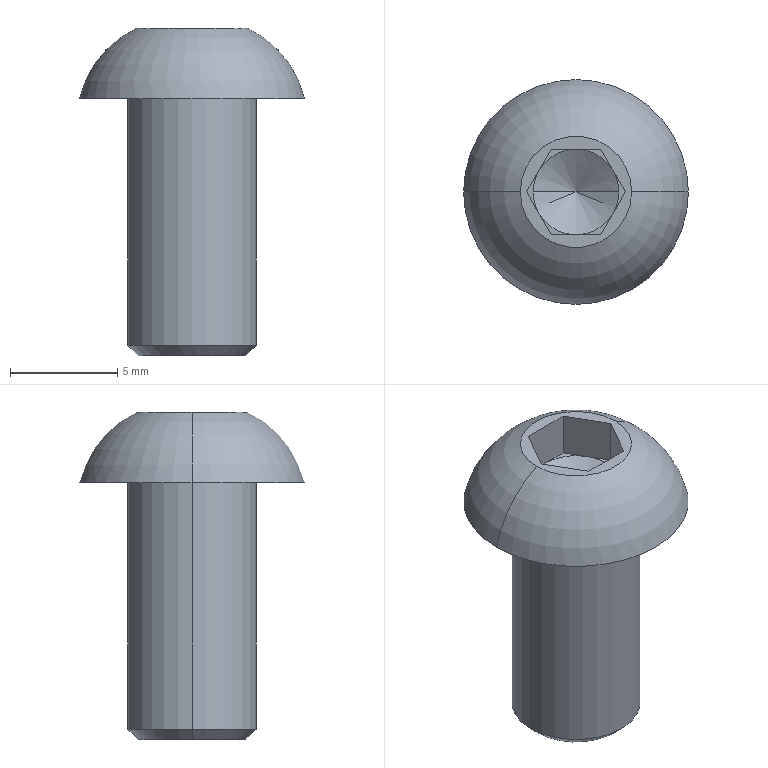Part | NX | features BREP 1 | 1 solid | 23 faces | box 10.5 x 10.5 x 15.3 mm | volume 504.847 mm3 | plane 15 | cone 4 | torus 2 | cylinder 2 | commonest cylinder face diameters 6 x2
STEP:
#1=CARTESIAN_POINT('',(0.,0.,0.0453));
#2=VERTEX_POINT('',#1);
#3=CARTESIAN_POINT('',(-2.,0.,1.2));
#4=VERTEX_POINT('',#3);
#5=CARTESIAN_POINT('',(-2.,0.,1.2));
#6=DIRECTION('',(-0.866,0.,0.5));
#7=VECTOR('',#6,1000.);
#8=LINE('',#5,#7);
#9=EDGE_CURVE('',#2,#4,#8,.T.);
#10=ORIENTED_EDGE('',*,*,#9,.F.);
#11=CARTESIAN_POINT('',(2.,0.,1.2));
#12=VERTEX_POINT('',#11);
#13=CARTESIAN_POINT('',(2.,0.,1.2));
#14=DIRECTION('',(0.866,0.,0.5));
#15=VECTOR('',#14,1000.);
#16=LINE('',#13,#15);
#17=EDGE_CURVE('',#2,#12,#16,.T.);
#18=ORIENTED_EDGE('',*,*,#17,.T.);
#19=CARTESIAN_POINT('',(1.732,1.,1.2));
#20=VERTEX_POINT('',#19);
#21=CARTESIAN_POINT('',(0.,0.,1.2));
#22=DIRECTION('',(0.,0.,1.));
#23=DIRECTION('',(1.,0.,0.));
#24=AXIS2_PLACEMENT_3D('',#21,#22,#23);
#25=CIRCLE('',#24,2.);
#26=EDGE_CURVE('',#12,#20,#25,.T.);
#27=ORIENTED_EDGE('',*,*,#26,.T.);
#28=CARTESIAN_POINT('',(0.,2.,1.2));
#29=VERTEX_POINT('',#28);
#30=CARTESIAN_POINT('',(0.,0.,1.2));
#31=DIRECTION('',(0.,0.,1.));
#32=DIRECTION('',(1.,0.,0.));
#33=AXIS2_PLACEMENT_3D('',#30,#31,#32);
#34=CIRCLE('',#33,2.);
#35=EDGE_CURVE('',#20,#29,#34,.T.);
#36=ORIENTED_EDGE('',*,*,#35,.T.);
#37=CARTESIAN_POINT('',(-1.732,1.,1.2));
#38=VERTEX_POINT('',#37);
#39=CARTESIAN_POINT('',(0.,0.,1.2));
#40=DIRECTION('',(0.,0.,-1.));
#41=DIRECTION('',(-1.,0.,0.));
#42=AXIS2_PLACEMENT_3D('',#39,#40,#41);
#43=CIRCLE('',#42,2.);
#44=EDGE_CURVE('',#38,#29,#43,.T.);
#45=ORIENTED_EDGE('',*,*,#44,.F.);
#46=CARTESIAN_POINT('',(0.,0.,1.2));
#47=DIRECTION('',(0.,0.,1.));
#48=DIRECTION('',(1.,0.,0.));
#49=AXIS2_PLACEMENT_3D('',#46,#47,#48);
#50=CIRCLE('',#49,2.);
#51=EDGE_CURVE('',#38,#4,#50,.T.);
#52=ORIENTED_EDGE('',*,*,#51,.T.);
#53=EDGE_LOOP('',(#10,#18,#27,#36,#45,#52));
#54=FACE_BOUND('',#53,.T.);
#55=CARTESIAN_POINT('',(0.,0.,1.2));
#56=DIRECTION('',(0.,0.,1.));
#57=DIRECTION('',(-1.,0.,0.));
#58=AXIS2_PLACEMENT_3D('',#55,#56,#57);
#59=CONICAL_SURFACE('',#58,2.,1.047);
#60=ADVANCED_FACE('',(#54),#59,.F.);
#61=CARTESIAN_POINT('',(-2.5,0.,-12.));
#62=VERTEX_POINT('',#61);
#63=CARTESIAN_POINT('',(2.5,0.,-12.));
#64=VERTEX_POINT('',#63);
#65=CARTESIAN_POINT('',(0.,0.,-12.));
#66=DIRECTION('',(0.,0.,1.));
#67=DIRECTION('',(-1.,0.,0.));
#68=AXIS2_PLACEMENT_3D('',#65,#66,#67);
#69=CIRCLE('',#68,2.5);
#70=EDGE_CURVE('',#62,#64,#69,.T.);
#71=ORIENTED_EDGE('',*,*,#70,.T.);
#72=CARTESIAN_POINT('',(3.,0.,-11.5));
#73=VERTEX_POINT('',#72);
#74=CARTESIAN_POINT('',(3.,0.,-11.5));
#75=DIRECTION('',(0.7071,0.,0.7071));
#76=VECTOR('',#75,1000.);
#77=LINE('',#74,#76);
#78=EDGE_CURVE('',#64,#73,#77,.T.);
#79=ORIENTED_EDGE('',*,*,#78,.T.);
#80=CARTESIAN_POINT('',(-3.,0.,-11.5));
#81=VERTEX_POINT('',#80);
#82=CARTESIAN_POINT('',(0.,0.,-11.5));
#83=DIRECTION('',(0.,0.,-1.));
#84=DIRECTION('',(-1.,0.,0.));
#85=AXIS2_PLACEMENT_3D('',#82,#83,#84);
#86=CIRCLE('',#85,3.);
#87=EDGE_CURVE('',#73,#81,#86,.T.);
#88=ORIENTED_EDGE('',*,*,#87,.T.);
#89=CARTESIAN_POINT('',(-3.,0.,-11.5));
#90=DIRECTION('',(-0.7071,0.,0.7071));
#91=VECTOR('',#90,1000.);
#92=LINE('',#89,#91);
#93=EDGE_CURVE('',#62,#81,#92,.T.);
#94=ORIENTED_EDGE('',*,*,#93,.F.);
#95=EDGE_LOOP('',(#71,#79,#88,#94));
#96=FACE_BOUND('',#95,.T.);
#97=CARTESIAN_POINT('',(0.,0.,-11.5));
#98=DIRECTION('',(0.,0.,1.));
#99=DIRECTION('',(-1.,0.,0.));
#100=AXIS2_PLACEMENT_3D('',#97,#98,#99);
#101=CONICAL_SURFACE('',#100,3.,0.7854);
#102=ADVANCED_FACE('',(#96),#101,.T.);
#103=CARTESIAN_POINT('',(5.25,0.,0.));
#104=VERTEX_POINT('',#103);
#105=CARTESIAN_POINT('',(-5.25,0.,0.));
#106=VERTEX_POINT('',#105);
#107=CARTESIAN_POINT('',(0.,0.,0.));
#108=DIRECTION('',(0.,0.,-1.));
#109=DIRECTION('',(-1.,0.,0.));
#110=AXIS2_PLACEMENT_3D('',#107,#108,#109);
#111=CIRCLE('',#110,5.25);
#112=EDGE_CURVE('',#104,#106,#111,.T.);
#113=ORIENTED_EDGE('',*,*,#112,.F.);
#114=CARTESIAN_POINT('',(2.6,0.,3.3));
#115=VERTEX_POINT('',#114);
#116=CARTESIAN_POINT('',(0.5657,0.,-1.048));
#117=DIRECTION('',(0.,-1.,0.));
#118=DIRECTION('',(1.,0.,0.));
#119=AXIS2_PLACEMENT_3D('',#116,#117,#118);
#120=CIRCLE('',#119,4.8);
#121=EDGE_CURVE('',#104,#115,#120,.T.);
#122=ORIENTED_EDGE('',*,*,#121,.T.);
#123=CARTESIAN_POINT('',(-2.6,0.,3.3));
#124=VERTEX_POINT('',#123);
#125=CARTESIAN_POINT('',(0.,0.,3.3));
#126=DIRECTION('',(0.,0.,-1.));
#127=DIRECTION('',(-1.,0.,0.));
#128=AXIS2_PLACEMENT_3D('',#125,#126,#127);
#129=CIRCLE('',#128,2.6);
#130=EDGE_CURVE('',#115,#124,#129,.T.);
#131=ORIENTED_EDGE('',*,*,#130,.T.);
#132=CARTESIAN_POINT('',(-0.5657,0.,-1.048));
#133=DIRECTION('',(0.,1.,0.));
#134=DIRECTION('',(0.,0.,1.));
#135=AXIS2_PLACEMENT_3D('',#132,#133,#134);
#136=CIRCLE('',#135,4.8);
#137=EDGE_CURVE('',#106,#124,#136,.T.);
#138=ORIENTED_EDGE('',*,*,#137,.F.);
#139=EDGE_LOOP('',(#113,#122,#131,#138));
#140=FACE_BOUND('',#139,.T.);
#141=CARTESIAN_POINT('',(0.,0.,-1.048));
#142=DIRECTION('',(0.,0.,1.));
#143=DIRECTION('',(-1.,0.,0.));
#144=AXIS2_PLACEMENT_3D('',#141,#142,#143);
#145=DEGENERATE_TOROIDAL_SURFACE('',#144,0.5657,4.8,.T.);
#146=ADVANCED_FACE('',(#140),#145,.T.);
#147=ORIENTED_EDGE('',*,*,#87,.F.);
#148=CARTESIAN_POINT('',(3.,0.,0.));
#149=VERTEX_POINT('',#148);
#150=CARTESIAN_POINT('',(3.,0.,-12.));
#151=DIRECTION('',(0.,0.,1.));
#152=VECTOR('',#151,1000.);
#153=LINE('',#150,#152);
#154=EDGE_CURVE('',#73,#149,#153,.T.);
#155=ORIENTED_EDGE('',*,*,#154,.T.);
#156=CARTESIAN_POINT('',(-3.,0.,0.));
#157=VERTEX_POINT('',#156);
#158=CARTESIAN_POINT('',(0.,0.,0.));
#159=DIRECTION('',(0.,0.,1.));
#160=DIRECTION('',(1.,0.,0.));
#161=AXIS2_PLACEMENT_3D('',#158,#159,#160);
#162=CIRCLE('',#161,3.);
#163=EDGE_CURVE('',#157,#149,#162,.T.);
#164=ORIENTED_EDGE('',*,*,#163,.F.);
#165=CARTESIAN_POINT('',(-3.,0.,-12.));
#166=DIRECTION('',(0.,0.,1.));
#167=VECTOR('',#166,1000.);
#168=LINE('',#165,#167);
#169=EDGE_CURVE('',#81,#157,#168,.T.);
#170=ORIENTED_EDGE('',*,*,#169,.F.);
#171=EDGE_LOOP('',(#147,#155,#164,#170));
#172=FACE_BOUND('',#171,.T.);
#173=CARTESIAN_POINT('',(0.,0.,-12.));
#174=DIRECTION('',(0.,0.,1.));
#175=DIRECTION('',(-1.,0.,0.));
#176=AXIS2_PLACEMENT_3D('',#173,#174,#175);
#177=CYLINDRICAL_SURFACE('',#176,3.);
#178=ADVANCED_FACE('',(#172),#177,.T.);
#179=CARTESIAN_POINT('',(1.155,2.,1.2));
#180=VERTEX_POINT('',#179);
#181=CARTESIAN_POINT('',(2.309,0.,1.2));
#182=DIRECTION('',(-0.5,0.866,0.));
#183=VECTOR('',#182,1000.);
#184=LINE('',#181,#183);
#185=EDGE_CURVE('',#20,#180,#184,.T.);
#186=ORIENTED_EDGE('',*,*,#185,.T.);
#187=CARTESIAN_POINT('',(1.155,2.,1.2));
#188=DIRECTION('',(-1.,0.,0.));
#189=VECTOR('',#188,1000.);
#190=LINE('',#187,#189);
#191=EDGE_CURVE('',#180,#29,#190,.T.);
#192=ORIENTED_EDGE('',*,*,#191,.T.);
#193=ORIENTED_EDGE('',*,*,#35,.F.);
#194=EDGE_LOOP('',(#186,#192,#193));
#195=FACE_BOUND('',#194,.T.);
#196=CARTESIAN_POINT('',(0.,0.,1.2));
#197=DIRECTION('',(0.,0.,-1.));
#198=DIRECTION('',(0.,-1.,0.));
#199=AXIS2_PLACEMENT_3D('',#196,#197,#198);
#200=PLANE('',#199);
#201=ADVANCED_FACE('',(#195),#200,.F.);
#202=CARTESIAN_POINT('',(-1.155,2.,1.2));
#203=VERTEX_POINT('',#202);
#204=CARTESIAN_POINT('',(1.155,2.,1.2));
#205=DIRECTION('',(-1.,0.,0.));
#206=VECTOR('',#205,1000.);
#207=LINE('',#204,#206);
#208=EDGE_CURVE('',#29,#203,#207,.T.);
#209=ORIENTED_EDGE('',*,*,#208,.T.);
#210=CARTESIAN_POINT('',(-1.155,2.,1.2));
#211=DIRECTION('',(-0.5,-0.866,0.));
#212=VECTOR('',#211,1000.);
#213=LINE('',#210,#212);
#214=EDGE_CURVE('',#203,#38,#213,.T.);
#215=ORIENTED_EDGE('',*,*,#214,.T.);
#216=ORIENTED_EDGE('',*,*,#44,.T.);
#217=EDGE_LOOP('',(#209,#215,#216));
#218=FACE_BOUND('',#217,.T.);
#219=CARTESIAN_POINT('',(0.,0.,1.2));
#220=DIRECTION('',(0.,0.,-1.));
#221=DIRECTION('',(0.,-1.,0.));
#222=AXIS2_PLACEMENT_3D('',#219,#220,#221);
#223=PLANE('',#222);
#224=ADVANCED_FACE('',(#218),#223,.F.);
#225=CARTESIAN_POINT('',(-2.309,0.,1.2));
#226=VERTEX_POINT('',#225);
#227=CARTESIAN_POINT('',(-1.155,2.,1.2));
#228=DIRECTION('',(-0.5,-0.866,0.));
#229=VECTOR('',#228,1000.);
#230=LINE('',#227,#229);
#231=EDGE_CURVE('',#38,#226,#230,.T.);
#232=ORIENTED_EDGE('',*,*,#231,.T.);
#233=CARTESIAN_POINT('',(-1.732,-1.,1.2));
#234=VERTEX_POINT('',#233);
#235=CARTESIAN_POINT('',(-2.309,0.,1.2));
#236=DIRECTION('',(0.5,-0.866,0.));
#237=VECTOR('',#236,1000.);
#238=LINE('',#235,#237);
#239=EDGE_CURVE('',#226,#234,#238,.T.);
#240=ORIENTED_EDGE('',*,*,#239,.T.);
#241=CARTESIAN_POINT('',(0.,0.,1.2));
#242=DIRECTION('',(0.,0.,1.));
#243=DIRECTION('',(1.,0.,0.));
#244=AXIS2_PLACEMENT_3D('',#241,#242,#243);
#245=CIRCLE('',#244,2.);
#246=EDGE_CURVE('',#4,#234,#245,.T.);
#247=ORIENTED_EDGE('',*,*,#246,.F.);
#248=ORIENTED_EDGE('',*,*,#51,.F.);
#249=EDGE_LOOP('',(#232,#240,#247,#248));
#250=FACE_BOUND('',#249,.T.);
#251=CARTESIAN_POINT('',(0.,0.,1.2));
#252=DIRECTION('',(0.,0.,-1.));
#253=DIRECTION('',(0.,-1.,0.));
#254=AXIS2_PLACEMENT_3D('',#251,#252,#253);
#255=PLANE('',#254);
#256=ADVANCED_FACE('',(#250),#255,.F.);
#257=CARTESIAN_POINT('',(-1.155,-2.,1.2));
#258=VERTEX_POINT('',#257);
#259=CARTESIAN_POINT('',(-2.309,0.,1.2));
#260=DIRECTION('',(0.5,-0.866,0.));
#261=VECTOR('',#260,1000.);
#262=LINE('',#259,#261);
#263=EDGE_CURVE('',#234,#258,#262,.T.);
#264=ORIENTED_EDGE('',*,*,#263,.T.);
#265=CARTESIAN_POINT('',(0.,-2.,1.2));
#266=VERTEX_POINT('',#265);
#267=CARTESIAN_POINT('',(-1.155,-2.,1.2));
#268=DIRECTION('',(1.,0.,0.));
#269=VECTOR('',#268,1000.);
#270=LINE('',#267,#269);
#271=EDGE_CURVE('',#258,#266,#270,.T.);
#272=ORIENTED_EDGE('',*,*,#271,.T.);
#273=CARTESIAN_POINT('',(0.,0.,1.2));
#274=DIRECTION('',(0.,0.,1.));
#275=DIRECTION('',(1.,0.,0.));
#276=AXIS2_PLACEMENT_3D('',#273,#274,#275);
#277=CIRCLE('',#276,2.);
#278=EDGE_CURVE('',#234,#266,#277,.T.);
#279=ORIENTED_EDGE('',*,*,#278,.F.);
#280=EDGE_LOOP('',(#264,#272,#279));
#281=FACE_BOUND('',#280,.T.);
#282=CARTESIAN_POINT('',(0.,0.,1.2));
#283=DIRECTION('',(0.,0.,-1.));
#284=DIRECTION('',(0.,-1.,0.));
#285=AXIS2_PLACEMENT_3D('',#282,#283,#284);
#286=PLANE('',#285);
#287=ADVANCED_FACE('',(#281),#286,.F.);
#288=CARTESIAN_POINT('',(1.155,-2.,1.2));
#289=VERTEX_POINT('',#288);
#290=CARTESIAN_POINT('',(-1.155,-2.,1.2));
#291=DIRECTION('',(1.,0.,0.));
#292=VECTOR('',#291,1000.);
#293=LINE('',#290,#292);
#294=EDGE_CURVE('',#266,#289,#293,.T.);
#295=ORIENTED_EDGE('',*,*,#294,.T.);
#296=CARTESIAN_POINT('',(1.732,-1.,1.2));
#297=VERTEX_POINT('',#296);
#298=CARTESIAN_POINT('',(1.155,-2.,1.2));
#299=DIRECTION('',(0.5,0.866,0.));
#300=VECTOR('',#299,1000.);
#301=LINE('',#298,#300);
#302=EDGE_CURVE('',#289,#297,#301,.T.);
#303=ORIENTED_EDGE('',*,*,#302,.T.);
#304=CARTESIAN_POINT('',(0.,0.,1.2));
#305=DIRECTION('',(0.,0.,1.));
#306=DIRECTION('',(1.,0.,0.));
#307=AXIS2_PLACEMENT_3D('',#304,#305,#306);
#308=CIRCLE('',#307,2.);
#309=EDGE_CURVE('',#266,#297,#308,.T.);
#310=ORIENTED_EDGE('',*,*,#309,.F.);
#311=EDGE_LOOP('',(#295,#303,#310));
#312=FACE_BOUND('',#311,.T.);
#313=CARTESIAN_POINT('',(0.,0.,1.2));
#314=DIRECTION('',(0.,0.,-1.));
#315=DIRECTION('',(0.,-1.,0.));
#316=AXIS2_PLACEMENT_3D('',#313,#314,#315);
#317=PLANE('',#316);
#318=ADVANCED_FACE('',(#312),#317,.F.);
#319=CARTESIAN_POINT('',(0.,0.,3.3));
#320=DIRECTION('',(0.,0.,-1.));
#321=DIRECTION('',(-1.,0.,0.));
#322=AXIS2_PLACEMENT_3D('',#319,#320,#321);
#323=CIRCLE('',#322,2.6);
#324=EDGE_CURVE('',#124,#115,#323,.T.);
#325=ORIENTED_EDGE('',*,*,#324,.F.);
#326=ORIENTED_EDGE('',*,*,#130,.F.);
#327=EDGE_LOOP('',(#325,#326));
#328=FACE_BOUND('',#327,.T.);
#329=CARTESIAN_POINT('',(2.309,0.,3.3));
#330=VERTEX_POINT('',#329);
#331=CARTESIAN_POINT('',(1.155,2.,3.3));
#332=VERTEX_POINT('',#331);
#333=CARTESIAN_POINT('',(2.309,0.,3.3));
#334=DIRECTION('',(-0.5,0.866,0.));
#335=VECTOR('',#334,1000.);
#336=LINE('',#333,#335);
#337=EDGE_CURVE('',#330,#332,#336,.T.);
#338=ORIENTED_EDGE('',*,*,#337,.F.);
#339=CARTESIAN_POINT('',(1.155,-2.,3.3));
#340=VERTEX_POINT('',#339);
#341=CARTESIAN_POINT('',(1.155,-2.,3.3));
#342=DIRECTION('',(0.5,0.866,0.));
#343=VECTOR('',#342,1000.);
#344=LINE('',#341,#343);
#345=EDGE_CURVE('',#340,#330,#344,.T.);
#346=ORIENTED_EDGE('',*,*,#345,.F.);
#347=CARTESIAN_POINT('',(-1.155,-2.,3.3));
#348=VERTEX_POINT('',#347);
#349=CARTESIAN_POINT('',(-1.155,-2.,3.3));
#350=DIRECTION('',(1.,0.,0.));
#351=VECTOR('',#350,1000.);
#352=LINE('',#349,#351);
#353=EDGE_CURVE('',#348,#340,#352,.T.);
#354=ORIENTED_EDGE('',*,*,#353,.F.);
#355=CARTESIAN_POINT('',(-2.309,0.,3.3));
#356=VERTEX_POINT('',#355);
#357=CARTESIAN_POINT('',(-2.309,0.,3.3));
#358=DIRECTION('',(0.5,-0.866,0.));
#359=VECTOR('',#358,1000.);
#360=LINE('',#357,#359);
#361=EDGE_CURVE('',#356,#348,#360,.T.);
#362=ORIENTED_EDGE('',*,*,#361,.F.);
#363=CARTESIAN_POINT('',(-1.155,2.,3.3));
#364=VERTEX_POINT('',#363);
#365=CARTESIAN_POINT('',(-1.155,2.,3.3));
#366=DIRECTION('',(-0.5,-0.866,0.));
#367=VECTOR('',#366,1000.);
#368=LINE('',#365,#367);
#369=EDGE_CURVE('',#364,#356,#368,.T.);
#370=ORIENTED_EDGE('',*,*,#369,.F.);
#371=CARTESIAN_POINT('',(1.155,2.,3.3));
#372=DIRECTION('',(-1.,0.,0.));
#373=VECTOR('',#372,1000.);
#374=LINE('',#371,#373);
#375=EDGE_CURVE('',#332,#364,#374,.T.);
#376=ORIENTED_EDGE('',*,*,#375,.F.);
#377=EDGE_LOOP('',(#338,#346,#354,#362,#370,#376));
#378=FACE_BOUND('',#377,.T.);
#379=CARTESIAN_POINT('',(0.,0.,3.3));
#380=DIRECTION('',(0.,0.,-1.));
#381=DIRECTION('',(0.,-1.,0.));
#382=AXIS2_PLACEMENT_3D('',#379,#380,#381);
#383=PLANE('',#382);
#384=ADVANCED_FACE('',(#328,#378),#383,.F.);
#385=CARTESIAN_POINT('',(0.,0.,0.));
#386=DIRECTION('',(0.,0.,-1.));
#387=DIRECTION('',(-1.,0.,0.));
#388=AXIS2_PLACEMENT_3D('',#385,#386,#387);
#389=CIRCLE('',#388,5.25);
#390=EDGE_CURVE('',#106,#104,#389,.T.);
#391=ORIENTED_EDGE('',*,*,#390,.T.);
#392=ORIENTED_EDGE('',*,*,#112,.T.);
#393=EDGE_LOOP('',(#391,#392));
#394=FACE_BOUND('',#393,.T.);
#395=ORIENTED_EDGE('',*,*,#163,.T.);
#396=CARTESIAN_POINT('',(0.,0.,0.));
#397=DIRECTION('',(0.,0.,1.));
#398=DIRECTION('',(1.,0.,0.));
#399=AXIS2_PLACEMENT_3D('',#396,#397,#398);
#400=CIRCLE('',#399,3.);
#401=EDGE_CURVE('',#149,#157,#400,.T.);
#402=ORIENTED_EDGE('',*,*,#401,.T.);
#403=EDGE_LOOP('',(#395,#402));
#404=FACE_BOUND('',#403,.T.);
#405=CARTESIAN_POINT('',(0.,0.,0.));
#406=DIRECTION('',(0.,0.,-1.));
#407=DIRECTION('',(0.,-1.,0.));
#408=AXIS2_PLACEMENT_3D('',#405,#406,#407);
#409=PLANE('',#408);
#410=ADVANCED_FACE('',(#394,#404),#409,.T.);
#411=ORIENTED_EDGE('',*,*,#154,.F.);
#412=CARTESIAN_POINT('',(0.,0.,-11.5));
#413=DIRECTION('',(0.,0.,-1.));
#414=DIRECTION('',(-1.,0.,0.));
#415=AXIS2_PLACEMENT_3D('',#412,#413,#414);
#416=CIRCLE('',#415,3.);
#417=EDGE_CURVE('',#81,#73,#416,.T.);
#418=ORIENTED_EDGE('',*,*,#417,.F.);
#419=ORIENTED_EDGE('',*,*,#169,.T.);
#420=ORIENTED_EDGE('',*,*,#401,.F.);
#421=EDGE_LOOP('',(#411,#418,#419,#420));
#422=FACE_BOUND('',#421,.T.);
#423=CARTESIAN_POINT('',(0.,0.,-12.));
#424=DIRECTION('',(0.,0.,1.));
#425=DIRECTION('',(-1.,0.,0.));
#426=AXIS2_PLACEMENT_3D('',#423,#424,#425);
#427=CYLINDRICAL_SURFACE('',#426,3.);
#428=ADVANCED_FACE('',(#422),#427,.T.);
#429=ORIENTED_EDGE('',*,*,#70,.F.);
#430=CARTESIAN_POINT('',(0.,0.,-12.));
#431=DIRECTION('',(0.,0.,1.));
#432=DIRECTION('',(-1.,0.,0.));
#433=AXIS2_PLACEMENT_3D('',#430,#431,#432);
#434=CIRCLE('',#433,2.5);
#435=EDGE_CURVE('',#64,#62,#434,.T.);
#436=ORIENTED_EDGE('',*,*,#435,.F.);
#437=EDGE_LOOP('',(#429,#436));
#438=FACE_BOUND('',#437,.T.);
#439=CARTESIAN_POINT('',(0.,0.,-12.));
#440=DIRECTION('',(0.,0.,1.));
#441=DIRECTION('',(1.,0.,0.));
#442=AXIS2_PLACEMENT_3D('',#439,#440,#441);
#443=PLANE('',#442);
#444=ADVANCED_FACE('',(#438),#443,.F.);
#445=ORIENTED_EDGE('',*,*,#121,.F.);
#446=ORIENTED_EDGE('',*,*,#390,.F.);
#447=ORIENTED_EDGE('',*,*,#137,.T.);
#448=ORIENTED_EDGE('',*,*,#324,.T.);
#449=EDGE_LOOP('',(#445,#446,#447,#448));
#450=FACE_BOUND('',#449,.T.);
#451=CARTESIAN_POINT('',(0.,0.,-1.048));
#452=DIRECTION('',(0.,0.,1.));
#453=DIRECTION('',(-1.,0.,0.));
#454=AXIS2_PLACEMENT_3D('',#451,#452,#453);
#455=DEGENERATE_TOROIDAL_SURFACE('',#454,0.5657,4.8,.T.);
#456=ADVANCED_FACE('',(#450),#455,.T.);
#457=ORIENTED_EDGE('',*,*,#78,.F.);
#458=ORIENTED_EDGE('',*,*,#435,.T.);
#459=ORIENTED_EDGE('',*,*,#93,.T.);
#460=ORIENTED_EDGE('',*,*,#417,.T.);
#461=EDGE_LOOP('',(#457,#458,#459,#460));
#462=FACE_BOUND('',#461,.T.);
#463=CARTESIAN_POINT('',(0.,0.,-11.5));
#464=DIRECTION('',(0.,0.,1.));
#465=DIRECTION('',(-1.,0.,0.));
#466=AXIS2_PLACEMENT_3D('',#463,#464,#465);
#467=CONICAL_SURFACE('',#466,3.,0.7854);
#468=ADVANCED_FACE('',(#462),#467,.T.);
#469=ORIENTED_EDGE('',*,*,#337,.T.);
#470=CARTESIAN_POINT('',(1.155,2.,1.2));
#471=DIRECTION('',(0.,0.,1.));
#472=VECTOR('',#471,1000.);
#473=LINE('',#470,#472);
#474=EDGE_CURVE('',#180,#332,#473,.T.);
#475=ORIENTED_EDGE('',*,*,#474,.F.);
#476=ORIENTED_EDGE('',*,*,#185,.F.);
#477=CARTESIAN_POINT('',(2.309,0.,1.2));
#478=VERTEX_POINT('',#477);
#479=CARTESIAN_POINT('',(2.309,0.,1.2));
#480=DIRECTION('',(-0.5,0.866,0.));
#481=VECTOR('',#480,1000.);
#482=LINE('',#479,#481);
#483=EDGE_CURVE('',#478,#20,#482,.T.);
#484=ORIENTED_EDGE('',*,*,#483,.F.);
#485=CARTESIAN_POINT('',(2.309,0.,1.2));
#486=DIRECTION('',(0.,0.,1.));
#487=VECTOR('',#486,1000.);
#488=LINE('',#485,#487);
#489=EDGE_CURVE('',#478,#330,#488,.T.);
#490=ORIENTED_EDGE('',*,*,#489,.T.);
#491=EDGE_LOOP('',(#469,#475,#476,#484,#490));
#492=FACE_BOUND('',#491,.T.);
#493=CARTESIAN_POINT('',(2.309,0.,1.2));
#494=DIRECTION('',(-0.866,-0.5,0.));
#495=DIRECTION('',(-0.5,0.866,0.));
#496=AXIS2_PLACEMENT_3D('',#493,#494,#495);
#497=PLANE('',#496);
#498=ADVANCED_FACE('',(#492),#497,.T.);
#499=ORIENTED_EDGE('',*,*,#375,.T.);
#500=CARTESIAN_POINT('',(-1.155,2.,1.2));
#501=DIRECTION('',(0.,0.,1.));
#502=VECTOR('',#501,1000.);
#503=LINE('',#500,#502);
#504=EDGE_CURVE('',#203,#364,#503,.T.);
#505=ORIENTED_EDGE('',*,*,#504,.F.);
#506=ORIENTED_EDGE('',*,*,#208,.F.);
#507=ORIENTED_EDGE('',*,*,#191,.F.);
#508=ORIENTED_EDGE('',*,*,#474,.T.);
#509=EDGE_LOOP('',(#499,#505,#506,#507,#508));
#510=FACE_BOUND('',#509,.T.);
#511=CARTESIAN_POINT('',(1.155,2.,1.2));
#512=DIRECTION('',(0.,-1.,0.));
#513=DIRECTION('',(0.,0.,-1.));
#514=AXIS2_PLACEMENT_3D('',#511,#512,#513);
#515=PLANE('',#514);
#516=ADVANCED_FACE('',(#510),#515,.T.);
#517=ORIENTED_EDGE('',*,*,#369,.T.);
#518=CARTESIAN_POINT('',(-2.309,0.,1.2));
#519=DIRECTION('',(0.,0.,1.));
#520=VECTOR('',#519,1000.);
#521=LINE('',#518,#520);
#522=EDGE_CURVE('',#226,#356,#521,.T.);
#523=ORIENTED_EDGE('',*,*,#522,.F.);
#524=ORIENTED_EDGE('',*,*,#231,.F.);
#525=ORIENTED_EDGE('',*,*,#214,.F.);
#526=ORIENTED_EDGE('',*,*,#504,.T.);
#527=EDGE_LOOP('',(#517,#523,#524,#525,#526));
#528=FACE_BOUND('',#527,.T.);
#529=CARTESIAN_POINT('',(-1.155,2.,1.2));
#530=DIRECTION('',(0.866,-0.5,0.));
#531=DIRECTION('',(0.,0.,-1.));
#532=AXIS2_PLACEMENT_3D('',#529,#530,#531);
#533=PLANE('',#532);
#534=ADVANCED_FACE('',(#528),#533,.T.);
#535=ORIENTED_EDGE('',*,*,#361,.T.);
#536=CARTESIAN_POINT('',(-1.155,-2.,1.2));
#537=DIRECTION('',(0.,0.,1.));
#538=VECTOR('',#537,1000.);
#539=LINE('',#536,#538);
#540=EDGE_CURVE('',#258,#348,#539,.T.);
#541=ORIENTED_EDGE('',*,*,#540,.F.);
#542=ORIENTED_EDGE('',*,*,#263,.F.);
#543=ORIENTED_EDGE('',*,*,#239,.F.);
#544=ORIENTED_EDGE('',*,*,#522,.T.);
#545=EDGE_LOOP('',(#535,#541,#542,#543,#544));
#546=FACE_BOUND('',#545,.T.);
#547=CARTESIAN_POINT('',(-2.309,0.,1.2));
#548=DIRECTION('',(0.866,0.5,0.));
#549=DIRECTION('',(0.,0.,-1.));
#550=AXIS2_PLACEMENT_3D('',#547,#548,#549);
#551=PLANE('',#550);
#552=ADVANCED_FACE('',(#546),#551,.T.);
#553=ORIENTED_EDGE('',*,*,#353,.T.);
#554=CARTESIAN_POINT('',(1.155,-2.,1.2));
#555=DIRECTION('',(0.,0.,1.));
#556=VECTOR('',#555,1000.);
#557=LINE('',#554,#556);
#558=EDGE_CURVE('',#289,#340,#557,.T.);
#559=ORIENTED_EDGE('',*,*,#558,.F.);
#560=ORIENTED_EDGE('',*,*,#294,.F.);
#561=ORIENTED_EDGE('',*,*,#271,.F.);
#562=ORIENTED_EDGE('',*,*,#540,.T.);
#563=EDGE_LOOP('',(#553,#559,#560,#561,#562));
#564=FACE_BOUND('',#563,.T.);
#565=CARTESIAN_POINT('',(-1.155,-2.,1.2));
#566=DIRECTION('',(0.,1.,0.));
#567=DIRECTION('',(1.,0.,0.));
#568=AXIS2_PLACEMENT_3D('',#565,#566,#567);
#569=PLANE('',#568);
#570=ADVANCED_FACE('',(#564),#569,.T.);
#571=ORIENTED_EDGE('',*,*,#345,.T.);
#572=ORIENTED_EDGE('',*,*,#489,.F.);
#573=CARTESIAN_POINT('',(1.155,-2.,1.2));
#574=DIRECTION('',(0.5,0.866,0.));
#575=VECTOR('',#574,1000.);
#576=LINE('',#573,#575);
#577=EDGE_CURVE('',#297,#478,#576,.T.);
#578=ORIENTED_EDGE('',*,*,#577,.F.);
#579=ORIENTED_EDGE('',*,*,#302,.F.);
#580=ORIENTED_EDGE('',*,*,#558,.T.);
#581=EDGE_LOOP('',(#571,#572,#578,#579,#580));
#582=FACE_BOUND('',#581,.T.);
#583=CARTESIAN_POINT('',(1.155,-2.,1.2));
#584=DIRECTION('',(-0.866,0.5,0.));
#585=DIRECTION('',(0.,0.,1.));
#586=AXIS2_PLACEMENT_3D('',#583,#584,#585);
#587=PLANE('',#586);
#588=ADVANCED_FACE('',(#582),#587,.T.);
#589=ORIENTED_EDGE('',*,*,#577,.T.);
#590=ORIENTED_EDGE('',*,*,#483,.T.);
#591=ORIENTED_EDGE('',*,*,#26,.F.);
#592=CARTESIAN_POINT('',(0.,0.,1.2));
#593=DIRECTION('',(0.,0.,1.));
#594=DIRECTION('',(1.,0.,0.));
#595=AXIS2_PLACEMENT_3D('',#592,#593,#594);
#596=CIRCLE('',#595,2.);
#597=EDGE_CURVE('',#297,#12,#596,.T.);
#598=ORIENTED_EDGE('',*,*,#597,.F.);
#599=EDGE_LOOP('',(#589,#590,#591,#598));
#600=FACE_BOUND('',#599,.T.);
#601=CARTESIAN_POINT('',(0.,0.,1.2));
#602=DIRECTION('',(0.,0.,-1.));
#603=DIRECTION('',(0.,-1.,0.));
#604=AXIS2_PLACEMENT_3D('',#601,#602,#603);
#605=PLANE('',#604);
#606=ADVANCED_FACE('',(#600),#605,.F.);
#607=ORIENTED_EDGE('',*,*,#17,.F.);
#608=ORIENTED_EDGE('',*,*,#9,.T.);
#609=ORIENTED_EDGE('',*,*,#246,.T.);
#610=ORIENTED_EDGE('',*,*,#278,.T.);
#611=ORIENTED_EDGE('',*,*,#309,.T.);
#612=ORIENTED_EDGE('',*,*,#597,.T.);
#613=EDGE_LOOP('',(#607,#608,#609,#610,#611,#612));
#614=FACE_BOUND('',#613,.T.);
#615=CARTESIAN_POINT('',(0.,0.,1.2));
#616=DIRECTION('',(0.,0.,1.));
#617=DIRECTION('',(-1.,0.,0.));
#618=AXIS2_PLACEMENT_3D('',#615,#616,#617);
#619=CONICAL_SURFACE('',#618,2.,1.047);
#620=ADVANCED_FACE('',(#614),#619,.F.);
#621=CLOSED_SHELL('',(#60,#102,#146,#178,#201,#224,#256,#287,#318,#384,#410,#428,#444,#456,#468,#498,#516,#534,#552,#570,#588,#606,#620));
#622=MANIFOLD_SOLID_BREP('',#621);
#623=(LENGTH_UNIT()NAMED_UNIT(*)SI_UNIT(.MILLI.,.METRE.));
#624=UNCERTAINTY_MEASURE_WITH_UNIT(LENGTH_MEASURE(0.00001),#623,'','');
#625=(NAMED_UNIT(*)PLANE_ANGLE_UNIT()SI_UNIT($,.RADIAN.));
#626=(NAMED_UNIT(*)SI_UNIT($,.STERADIAN.)SOLID_ANGLE_UNIT());
#627=(GEOMETRIC_REPRESENTATION_CONTEXT(3)GLOBAL_UNCERTAINTY_ASSIGNED_CONTEXT((#624))GLOBAL_UNIT_ASSIGNED_CONTEXT((#623,#625,#626))REPRESENTATION_CONTEXT('',''));
#628=ADVANCED_BREP_SHAPE_REPRESENTATION('',(#622),#627);